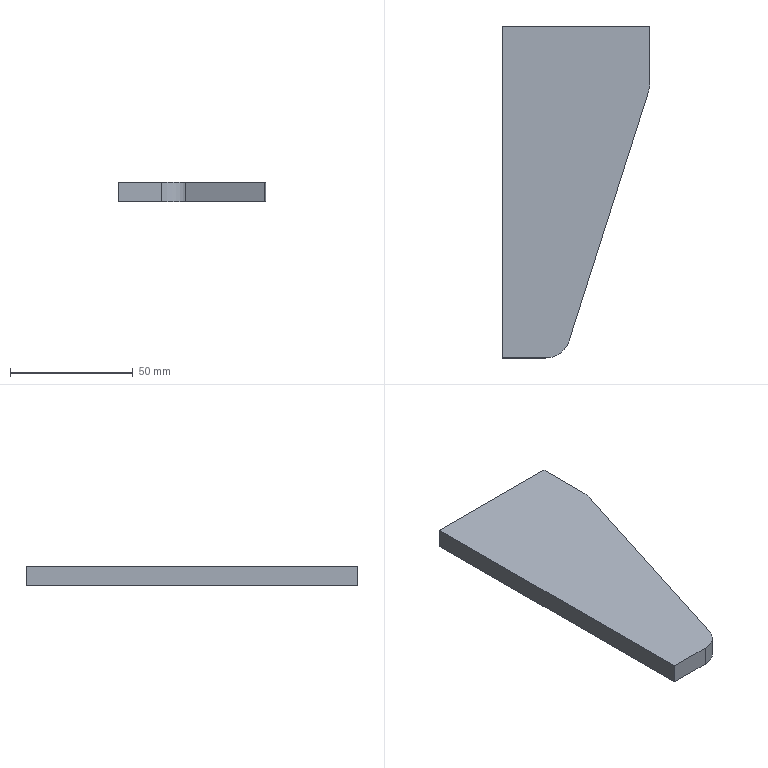Part | SolidWorks | features FlatPattern 1, SMBaseFlange 1, SheetMetal 1 | 1 solid | 9 faces | box 60 x 135 x 8 mm | volume 49319 mm3 | plane 7 | cylinder 2 | commonest cylinder face diameters 20 x2
STEP:
#1=CARTESIAN_POINT('',(56.899,-990.506,0.));
#2=VERTEX_POINT('',#1);
#3=CARTESIAN_POINT('',(56.899,-1125.506,0.));
#4=VERTEX_POINT('',#3);
#5=CARTESIAN_POINT('',(56.899,-1125.506,0.));
#6=DIRECTION('',(0.,-1.,0.));
#7=VECTOR('',#6,1000.);
#8=LINE('',#5,#7);
#9=EDGE_CURVE('',#2,#4,#8,.T.);
#10=ORIENTED_EDGE('',*,*,#9,.F.);
#11=CARTESIAN_POINT('',(56.899,-990.506,-8.));
#12=VERTEX_POINT('',#11);
#13=CARTESIAN_POINT('',(56.899,-990.506,-8.));
#14=DIRECTION('',(0.,0.,1.));
#15=VECTOR('',#14,1000.);
#16=LINE('',#13,#15);
#17=EDGE_CURVE('',#12,#2,#16,.T.);
#18=ORIENTED_EDGE('',*,*,#17,.F.);
#19=CARTESIAN_POINT('',(56.899,-1125.506,-8.));
#20=VERTEX_POINT('',#19);
#21=CARTESIAN_POINT('',(56.899,-1125.506,-8.));
#22=DIRECTION('',(0.,-1.,0.));
#23=VECTOR('',#22,1000.);
#24=LINE('',#21,#23);
#25=EDGE_CURVE('',#12,#20,#24,.T.);
#26=ORIENTED_EDGE('',*,*,#25,.T.);
#27=CARTESIAN_POINT('',(56.899,-1125.506,-8.));
#28=DIRECTION('',(0.,0.,1.));
#29=VECTOR('',#28,1000.);
#30=LINE('',#27,#29);
#31=EDGE_CURVE('',#20,#4,#30,.T.);
#32=ORIENTED_EDGE('',*,*,#31,.T.);
#33=EDGE_LOOP('',(#10,#18,#26,#32));
#34=FACE_OUTER_BOUND('',#33,.T.);
#35=CARTESIAN_POINT('',(56.899,-1125.506,-8.));
#36=DIRECTION('',(-1.,0.,0.));
#37=DIRECTION('',(0.,0.,1.));
#38=AXIS2_PLACEMENT_3D('',#35,#36,#37);
#39=PLANE('',#38);
#40=ADVANCED_FACE('',(#34),#39,.T.);
#41=CARTESIAN_POINT('',(116.899,-990.506,0.));
#42=VERTEX_POINT('',#41);
#43=CARTESIAN_POINT('',(56.899,-990.506,0.));
#44=DIRECTION('',(-1.,0.,0.));
#45=VECTOR('',#44,1000.);
#46=LINE('',#43,#45);
#47=EDGE_CURVE('',#42,#2,#46,.T.);
#48=ORIENTED_EDGE('',*,*,#47,.F.);
#49=CARTESIAN_POINT('',(116.899,-990.506,-8.));
#50=VERTEX_POINT('',#49);
#51=CARTESIAN_POINT('',(116.899,-990.506,-8.));
#52=DIRECTION('',(0.,0.,1.));
#53=VECTOR('',#52,1000.);
#54=LINE('',#51,#53);
#55=EDGE_CURVE('',#50,#42,#54,.T.);
#56=ORIENTED_EDGE('',*,*,#55,.F.);
#57=CARTESIAN_POINT('',(56.899,-990.506,-8.));
#58=DIRECTION('',(-1.,0.,0.));
#59=VECTOR('',#58,1000.);
#60=LINE('',#57,#59);
#61=EDGE_CURVE('',#50,#12,#60,.T.);
#62=ORIENTED_EDGE('',*,*,#61,.T.);
#63=ORIENTED_EDGE('',*,*,#17,.T.);
#64=EDGE_LOOP('',(#48,#56,#62,#63));
#65=FACE_OUTER_BOUND('',#64,.T.);
#66=CARTESIAN_POINT('',(56.899,-990.506,-8.));
#67=DIRECTION('',(0.,1.,0.));
#68=DIRECTION('',(-1.,0.,0.));
#69=AXIS2_PLACEMENT_3D('',#66,#67,#68);
#70=PLANE('',#69);
#71=ADVANCED_FACE('',(#65),#70,.T.);
#72=CARTESIAN_POINT('',(116.899,-1013.953,0.));
#73=VERTEX_POINT('',#72);
#74=CARTESIAN_POINT('',(116.899,-990.506,0.));
#75=DIRECTION('',(0.,1.,0.));
#76=VECTOR('',#75,1000.);
#77=LINE('',#74,#76);
#78=EDGE_CURVE('',#73,#42,#77,.T.);
#79=ORIENTED_EDGE('',*,*,#78,.F.);
#80=CARTESIAN_POINT('',(116.899,-1013.953,-8.));
#81=VERTEX_POINT('',#80);
#82=CARTESIAN_POINT('',(116.899,-1013.953,-8.));
#83=DIRECTION('',(0.,0.,1.));
#84=VECTOR('',#83,1000.);
#85=LINE('',#82,#84);
#86=EDGE_CURVE('',#81,#73,#85,.T.);
#87=ORIENTED_EDGE('',*,*,#86,.F.);
#88=CARTESIAN_POINT('',(116.899,-990.506,-8.));
#89=DIRECTION('',(0.,1.,0.));
#90=VECTOR('',#89,1000.);
#91=LINE('',#88,#90);
#92=EDGE_CURVE('',#81,#50,#91,.T.);
#93=ORIENTED_EDGE('',*,*,#92,.T.);
#94=ORIENTED_EDGE('',*,*,#55,.T.);
#95=EDGE_LOOP('',(#79,#87,#93,#94));
#96=FACE_OUTER_BOUND('',#95,.T.);
#97=CARTESIAN_POINT('',(116.899,-990.506,-8.));
#98=DIRECTION('',(1.,0.,0.));
#99=DIRECTION('',(0.,0.,-1.));
#100=AXIS2_PLACEMENT_3D('',#97,#98,#99);
#101=PLANE('',#100);
#102=ADVANCED_FACE('',(#96),#101,.T.);
#103=CARTESIAN_POINT('',(116.428,-1016.985,0.));
#104=VERTEX_POINT('',#103);
#105=CARTESIAN_POINT('',(106.899,-1013.953,0.));
#106=DIRECTION('',(0.,0.,1.));
#107=DIRECTION('',(-1.,0.,0.));
#108=AXIS2_PLACEMENT_3D('',#105,#106,#107);
#109=CIRCLE('',#108,10.);
#110=EDGE_CURVE('',#104,#73,#109,.T.);
#111=ORIENTED_EDGE('',*,*,#110,.F.);
#112=CARTESIAN_POINT('',(116.428,-1016.985,-8.));
#113=VERTEX_POINT('',#112);
#114=CARTESIAN_POINT('',(116.428,-1016.985,-8.));
#115=DIRECTION('',(0.,0.,1.));
#116=VECTOR('',#115,1000.);
#117=LINE('',#114,#116);
#118=EDGE_CURVE('',#113,#104,#117,.T.);
#119=ORIENTED_EDGE('',*,*,#118,.F.);
#120=CARTESIAN_POINT('',(106.899,-1013.953,-8.));
#121=DIRECTION('',(0.,0.,1.));
#122=DIRECTION('',(-1.,0.,0.));
#123=AXIS2_PLACEMENT_3D('',#120,#121,#122);
#124=CIRCLE('',#123,10.);
#125=EDGE_CURVE('',#113,#81,#124,.T.);
#126=ORIENTED_EDGE('',*,*,#125,.T.);
#127=ORIENTED_EDGE('',*,*,#86,.T.);
#128=EDGE_LOOP('',(#111,#119,#126,#127));
#129=FACE_OUTER_BOUND('',#128,.T.);
#130=CARTESIAN_POINT('',(106.899,-1013.953,-8.));
#131=DIRECTION('',(0.,0.,1.));
#132=DIRECTION('',(1.,0.,0.));
#133=AXIS2_PLACEMENT_3D('',#130,#131,#132);
#134=CYLINDRICAL_SURFACE('',#133,10.);
#135=ADVANCED_FACE('',(#129),#134,.T.);
#136=CARTESIAN_POINT('',(84.116,-1118.538,0.));
#137=VERTEX_POINT('',#136);
#138=CARTESIAN_POINT('',(116.428,-1016.985,0.));
#139=DIRECTION('',(0.3032,0.9529,0.));
#140=VECTOR('',#139,1000.);
#141=LINE('',#138,#140);
#142=EDGE_CURVE('',#137,#104,#141,.T.);
#143=ORIENTED_EDGE('',*,*,#142,.F.);
#144=CARTESIAN_POINT('',(84.116,-1118.538,-8.));
#145=VERTEX_POINT('',#144);
#146=CARTESIAN_POINT('',(84.116,-1118.538,-8.));
#147=DIRECTION('',(0.,0.,1.));
#148=VECTOR('',#147,1000.);
#149=LINE('',#146,#148);
#150=EDGE_CURVE('',#145,#137,#149,.T.);
#151=ORIENTED_EDGE('',*,*,#150,.F.);
#152=CARTESIAN_POINT('',(116.428,-1016.985,-8.));
#153=DIRECTION('',(0.3032,0.9529,0.));
#154=VECTOR('',#153,1000.);
#155=LINE('',#152,#154);
#156=EDGE_CURVE('',#145,#113,#155,.T.);
#157=ORIENTED_EDGE('',*,*,#156,.T.);
#158=ORIENTED_EDGE('',*,*,#118,.T.);
#159=EDGE_LOOP('',(#143,#151,#157,#158));
#160=FACE_OUTER_BOUND('',#159,.T.);
#161=CARTESIAN_POINT('',(116.428,-1016.985,-8.));
#162=DIRECTION('',(0.9529,-0.3032,0.));
#163=DIRECTION('',(0.3032,0.9529,0.));
#164=AXIS2_PLACEMENT_3D('',#161,#162,#163);
#165=PLANE('',#164);
#166=ADVANCED_FACE('',(#160),#165,.T.);
#167=CARTESIAN_POINT('',(74.587,-1125.506,0.));
#168=VERTEX_POINT('',#167);
#169=CARTESIAN_POINT('',(74.587,-1115.506,0.));
#170=DIRECTION('',(0.,0.,1.));
#171=DIRECTION('',(-1.,0.,0.));
#172=AXIS2_PLACEMENT_3D('',#169,#170,#171);
#173=CIRCLE('',#172,10.);
#174=EDGE_CURVE('',#168,#137,#173,.T.);
#175=ORIENTED_EDGE('',*,*,#174,.F.);
#176=CARTESIAN_POINT('',(74.587,-1125.506,-8.));
#177=VERTEX_POINT('',#176);
#178=CARTESIAN_POINT('',(74.587,-1125.506,-8.));
#179=DIRECTION('',(0.,0.,1.));
#180=VECTOR('',#179,1000.);
#181=LINE('',#178,#180);
#182=EDGE_CURVE('',#177,#168,#181,.T.);
#183=ORIENTED_EDGE('',*,*,#182,.F.);
#184=CARTESIAN_POINT('',(74.587,-1115.506,-8.));
#185=DIRECTION('',(0.,0.,1.));
#186=DIRECTION('',(-1.,0.,0.));
#187=AXIS2_PLACEMENT_3D('',#184,#185,#186);
#188=CIRCLE('',#187,10.);
#189=EDGE_CURVE('',#177,#145,#188,.T.);
#190=ORIENTED_EDGE('',*,*,#189,.T.);
#191=ORIENTED_EDGE('',*,*,#150,.T.);
#192=EDGE_LOOP('',(#175,#183,#190,#191));
#193=FACE_OUTER_BOUND('',#192,.T.);
#194=CARTESIAN_POINT('',(74.587,-1115.506,-8.));
#195=DIRECTION('',(0.,0.,1.));
#196=DIRECTION('',(1.,0.,0.));
#197=AXIS2_PLACEMENT_3D('',#194,#195,#196);
#198=CYLINDRICAL_SURFACE('',#197,10.);
#199=ADVANCED_FACE('',(#193),#198,.T.);
#200=CARTESIAN_POINT('',(74.587,-1125.506,0.));
#201=DIRECTION('',(1.,0.,0.));
#202=VECTOR('',#201,1000.);
#203=LINE('',#200,#202);
#204=EDGE_CURVE('',#4,#168,#203,.T.);
#205=ORIENTED_EDGE('',*,*,#204,.F.);
#206=ORIENTED_EDGE('',*,*,#31,.F.);
#207=CARTESIAN_POINT('',(74.587,-1125.506,-8.));
#208=DIRECTION('',(1.,0.,0.));
#209=VECTOR('',#208,1000.);
#210=LINE('',#207,#209);
#211=EDGE_CURVE('',#20,#177,#210,.T.);
#212=ORIENTED_EDGE('',*,*,#211,.T.);
#213=ORIENTED_EDGE('',*,*,#182,.T.);
#214=EDGE_LOOP('',(#205,#206,#212,#213));
#215=FACE_OUTER_BOUND('',#214,.T.);
#216=CARTESIAN_POINT('',(74.587,-1125.506,-8.));
#217=DIRECTION('',(0.,-1.,0.));
#218=DIRECTION('',(0.,0.,-1.));
#219=AXIS2_PLACEMENT_3D('',#216,#217,#218);
#220=PLANE('',#219);
#221=ADVANCED_FACE('',(#215),#220,.T.);
#222=ORIENTED_EDGE('',*,*,#25,.F.);
#223=ORIENTED_EDGE('',*,*,#61,.F.);
#224=ORIENTED_EDGE('',*,*,#92,.F.);
#225=ORIENTED_EDGE('',*,*,#125,.F.);
#226=ORIENTED_EDGE('',*,*,#156,.F.);
#227=ORIENTED_EDGE('',*,*,#189,.F.);
#228=ORIENTED_EDGE('',*,*,#211,.F.);
#229=EDGE_LOOP('',(#222,#223,#224,#225,#226,#227,#228));
#230=FACE_OUTER_BOUND('',#229,.T.);
#231=CARTESIAN_POINT('',(106.899,-1013.953,-8.));
#232=DIRECTION('',(0.,0.,-1.));
#233=DIRECTION('',(-1.,0.,0.));
#234=AXIS2_PLACEMENT_3D('',#231,#232,#233);
#235=PLANE('',#234);
#236=ADVANCED_FACE('',(#230),#235,.T.);
#237=ORIENTED_EDGE('',*,*,#9,.T.);
#238=ORIENTED_EDGE('',*,*,#204,.T.);
#239=ORIENTED_EDGE('',*,*,#174,.T.);
#240=ORIENTED_EDGE('',*,*,#142,.T.);
#241=ORIENTED_EDGE('',*,*,#110,.T.);
#242=ORIENTED_EDGE('',*,*,#78,.T.);
#243=ORIENTED_EDGE('',*,*,#47,.T.);
#244=EDGE_LOOP('',(#237,#238,#239,#240,#241,#242,#243));
#245=FACE_OUTER_BOUND('',#244,.T.);
#246=CARTESIAN_POINT('',(106.899,-1013.953,0.));
#247=DIRECTION('',(0.,0.,-1.));
#248=DIRECTION('',(-1.,0.,0.));
#249=AXIS2_PLACEMENT_3D('',#246,#247,#248);
#250=PLANE('',#249);
#251=ADVANCED_FACE('',(#245),#250,.F.);
#252=CLOSED_SHELL('',(#40,#71,#102,#135,#166,#199,#221,#236,#251));
#253=MANIFOLD_SOLID_BREP('',#252);
#254=CARTESIAN_POINT('',(0.,0.,0.));
#255=DIRECTION('',(0.,0.,1.));
#256=DIRECTION('',(1.,0.,0.));
#257=AXIS2_PLACEMENT_3D('',#254,#255,#256);
#258=(LENGTH_UNIT()NAMED_UNIT(*)SI_UNIT(.MILLI.,.METRE.));
#259=UNCERTAINTY_MEASURE_WITH_UNIT(LENGTH_MEASURE(0.00001),#258,'','');
#260=(NAMED_UNIT(*)PLANE_ANGLE_UNIT()SI_UNIT($,.RADIAN.));
#261=(NAMED_UNIT(*)SI_UNIT($,.STERADIAN.)SOLID_ANGLE_UNIT());
#262=(GEOMETRIC_REPRESENTATION_CONTEXT(3)GLOBAL_UNCERTAINTY_ASSIGNED_CONTEXT((#259))GLOBAL_UNIT_ASSIGNED_CONTEXT((#258,#260,#261))REPRESENTATION_CONTEXT('',''));
#263=ADVANCED_BREP_SHAPE_REPRESENTATION('',(#253,#257),#262);